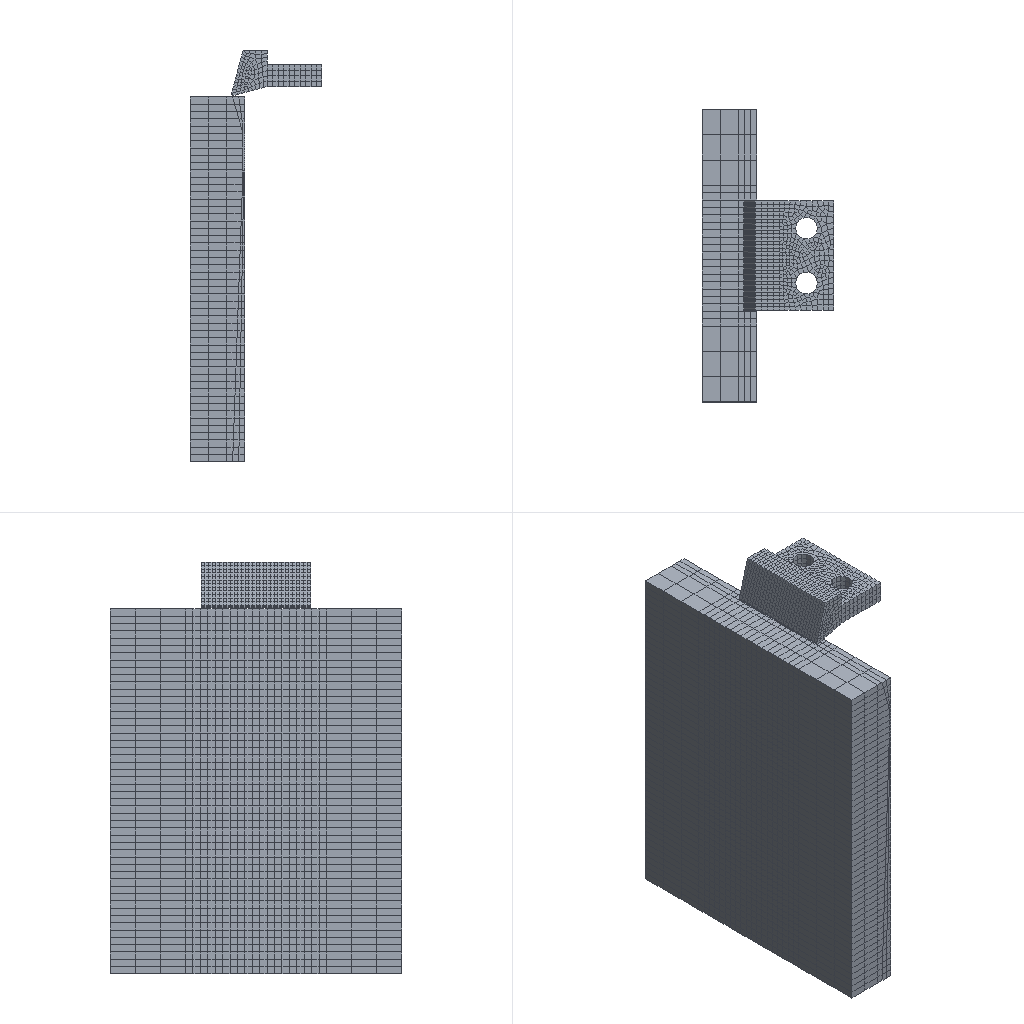Simulation study | abaqus
Set-up summary:
category,name,step,type,value,unit,region
solver,abaqus
solver,version,,,Abaqus/Explicit 2020
units,not stated in the deck,,not stated
analysis,deck,,transient,transient
load_step,Step-1,Step-1,transient
load_step,requested,,,1
mesh,nodes,,,19292
mesh,elements,,,12938
element_type,C3D8,,solid,3738
element_type,C3D8R,,solid,9200
load,load commands in deck,,count,1
bc,support commands in deck,,count,8
material,Q345,,in results
material,SLPSB,,in results
material,SLPSB2,,in results
material,SOIL,,in results
material,SOIL-COPY,,in results
check,setup vs results,,match,"per instance, exact: element labels, types and connectivity; labels of the nodes the elements use; coordinates of those nodes at DOUBLE_PRECISION in 1 of 3 instance(s)"
Abaqus input file, long lists of numbers shortened:
*Heading
** Job name: retiaoshi Model name: Model-1
** Generated by: Abaqus/CAE 2020
*Preprint, echo=NO, model=NO, history=NO, contact=NO
**
** PARTS
**
*Part, name=newwork
*Node
      1,           0.,  -59.32,         -20.
      2,         14.5,  -59.32,         -20.
** (7746 more lines like these left out)
*Element, type=C3D8R
 1,   74,  855, 3789,  839,    1,   53,  831,   59
 2,  855,  856, 3790, 3789,   53,   54,  832,  831
** (5998 more lines like these left out)
*Nset, nset=Set-7, generate
    1,  7748,     1
*Elset, elset=Set-7, generate
    1,  6000,     1
*Nset, nset=tuchipaa
   89,   90,   91,   92,   93,   94,   95,   96,   97,   98,   99,  100,  101,  102,  103,  104
  105,  106,  127,  128,  129,  130,  131,  132,  133,  134,  135,  136,  137,  138,  139,  140
** (219 more lines like these left out)
*Nset, nset=cc1
    4,    9,   16,   29,   30,   34,   43,   51,   56,   63,  172,  173,  545,  546,  559,  560
  603,  626,  709,  755, 1092, 3189, 3285, 3566
*Elset, elset=_tuti_S1, internal, generate
 4761,  4775,     1
*Elset, elset=_tuti_S4, internal, generate
  3,  45,   3
*Surface, type=ELEMENT, name=tuti
_tuti_S1, S1
_tuti_S4, S4
*Elset, elset=_m1_S1, internal, generate
 4761,  4775,     1
*Elset, elset=_m1_S4, internal, generate
  3,  45,   3
*Surface, type=ELEMENT, name=m1
_m1_S1, S1
_m1_S4, S4
** Section: tuti
*Solid Section, elset=Set-7, material=soil
,
*End Part
**
*Part, name=qiedao
*Node
      1,           3.,   7.052,           0.
      2,          -3.,   7.052,           0.
** (4779 more lines like these left out)
*Element, type=C3D8
   1,  408,  428,  429,  410, 2071, 2091, 2092, 2073
   2,   42,   41,    5,    6, 1026, 1027,  196,  138
** (3736 more lines like these left out)
*Node
   4782, 1.55431223e-15,   7.052,          15.
*Nset, nset=qiedao-RefPt_, internal
4782,
*Nset, nset=_PickedSet2, internal, generate
    1,  4781,     1
*Elset, elset=_PickedSet2, internal, generate
    1,  3738,     1
*Nset, nset=Set-daoju, generate
    1,  4782,     1
*Elset, elset=Set-daoju, generate
    1,  3738,     1
*Elset, elset=ganggang
    1,    2,    3,    4,    5,    6,    7,    8,    9,   10,   11,   12,   13,   14,   15,   16
   17,   18,   19,   20,   21,   22,   23,   24,   25,   26,   27,   28,   29,   30,   31,   32
** (104 more lines like these left out)
*Elset, elset=_keng-dao_S1, internal
    1,    2,    3,    4,    5,    6,    7,    8,    9,   10,   11,   12,   13,   14,   15,   16
   17,   18,   19,   20,   21,   22,   23,   24,   25,   26,   27,   28,   29,   30,   31,   32
** (22 more lines like these left out)
*Elset, elset=_keng-dao_S2, internal
 2524, 2525, 2526, 2527, 2528, 2529, 2530, 2531, 2532, 2533, 2534, 2535, 2536, 2537, 2538, 2539
 2540, 2541, 2542, 2543, 2544, 2545, 2546, 2547, 2548, 2549, 2550, 2551, 2552, 2553, 2554, 2555
** (22 more lines like these left out)
*Elset, elset=_keng-dao_S3, internal
    2,    5,    7,   10,   11,   12,   13,   16,   18,   21,   27,   28,   36,   89,   92,   94
   97,   98,   99,  100,  103,  105,  108,  114,  115,  123,  176,  179,  181,  184,  185,  186
** (29 more lines like these left out)
*Elset, elset=_keng-dao_S4, internal
    2,   89,  176,  263,  350,  437,  524,  611,  698,  785,  872,  959, 1046, 1133, 1220, 1307
 1394, 1481, 1568, 1655, 1742, 1829, 1916, 2003, 2090, 2177, 2264, 2351, 2438, 2525, 2640, 2722
** (3 more lines like these left out)
*Elset, elset=_keng-dao_S5, internal
    3,    8,   14,   15,   17,   19,   25,   29,   30,   31,   39,   41,   42,   44,   90,   95
  101,  102,  104,  106,  112,  116,  117,  118,  126,  128,  129,  131,  177,  182,  188,  189
** (30 more lines like these left out)
*Elset, elset=_keng-dao_S6, internal
    2,    8,   22,   84,   89,   95,  109,  171,  176,  182,  196,  258,  263,  269,  283,  345
  350,  356,  370,  432,  437,  443,  457,  519,  524,  530,  544,  606,  611,  617,  631,  693
** (9 more lines like these left out)
*Surface, type=ELEMENT, name=keng-dao
_keng-dao_S1, S1
_keng-dao_S2, S2
_keng-dao_S4, S4
_keng-dao_S6, S6
_keng-dao_S3, S3
_keng-dao_S5, S5
** Section: Q345
*Solid Section, elset=_PickedSet2, material=q345
,
*End Part
**
*Part, name=suliao
*Node
      1,           0.,         -80.,         -10.
      2,           0.,        -79.5,         -10.
** (6760 more lines like these left out)
*Element, type=C3D8R
   1,  323,  324,  485,  484,    1,    2,  163,  162
   2,  324,  325,  486,  485,    2,    3,  164,  163
** (3198 more lines like these left out)
*Nset, nset=Set-3, generate
    1,  6762,     1
*Elset, elset=Set-3, generate
    1,  3200,     1
*Nset, nset=suchipaa
   45,   46,   47,   48,   49,   50,   51,   52,   53,   54,   55,   56,   57,   58,   59,   60
   61,   62,   63,   64,   65,   66,   67,   68,   69,   70,   71,   72,   73,   74,   75,   76
** (166 more lines like these left out)
*Nset, nset=m2
    1,    2,    3,    4,    5,    6,    7,    8,    9,   10,   11,   12,   13,   14,   15,   16
   17,   18,   19,  140,  141,  142,  143,  144,  145,  146,  147,  148,  149,  150,  151,  152
** (51 more lines like these left out)
*Nset, nset=ce1
   1,   2,   3,   4,   5,   6,   7,   8,   9, 151, 152, 153, 154, 155, 156, 157
 158, 159, 160, 161, 162, 163, 164, 165, 166, 167, 168, 169, 170, 312, 313, 314
** (1 more lines like these left out)
*Nset, nset=ce2
 6441, 6442, 6443, 6444, 6445, 6446, 6447, 6448, 6449, 6592, 6593, 6594, 6595, 6596, 6597, 6598
 6599, 6600, 6601, 6602, 6603, 6604, 6605, 6606, 6607, 6608, 6609, 6610, 6753, 6754, 6755, 6756
** (1 more lines like these left out)
*Elset, elset=_suliaoban_S3, internal, generate
    1,  3200,     1
*Surface, type=ELEMENT, name=suliaoban
_suliaoban_S3, S3
** Section: suliaoti
*Solid Section, elset=Set-3, material=slpsb
,
*End Part
**
**
** ASSEMBLY
**
*Assembly, name=Assembly
**
*Instance, name=qiedao-1, part=qiedao
   28.199,         -55., 5.826
   28.199,         -55., 5.826, 27.621, -54.423, 6.403,         120.
*End Instance
**
*Instance, name=newwork-1, part=newwork
*End Instance
**
*Instance, name=suliao-1, part=suliao
        14.5,           0.,         -10.
*End Instance
**
*Nset, nset=Set-20, instance=qiedao-1
 4782,
*Nset, nset=Set-25, instance=suliao-1
    1,  161,  162,  322,  323,  483,  484,  644,  645,  805,  806,  966,  967, 1127, 1128, 1288
 1289, 1449, 1450, 1610, 1611, 1771, 1772, 1932, 1933, 2093, 2094, 2254, 2255, 2415, 2416, 2576
** (4 more lines like these left out)
*Elset, elset=Set-25, instance=suliao-1
    1,  160,  161,  320,  321,  480,  481,  640,  641,  800,  801,  960,  961, 1120, 1121, 1280
 1281, 1440, 1441, 1600, 1601, 1760, 1761, 1920, 1921, 2080, 2081, 2240, 2241, 2400, 2401, 2560
** (1 more lines like these left out)
*Nset, nset=Set-26, instance=newwork-1
    1,    5,    6,   10,   11,   13,   21,   22,   26,   27,   28,   39,   40,   42,   47,   50
   58,   59,   65,   66,   67,   68,   69,   70,   71,   72,   73,   74,  107,  108,  109,  110
** (81 more lines like these left out)
*Elset, elset=Set-26, instance=newwork-1
    1,    4,    7,   10,   13,   16,   19,   22,   25,   28,   31,   34,   37,   40,   43,   46
   49,   52,   55,   58,   61,   64,   67,   70,   73,   76,   79,   82,   85,   88,   91,   94
** (77 more lines like these left out)
*Nset, nset=_PickedSet56, internal, instance=qiedao-1
 4782,
*Surface, type=NODE, name=newwork-1_tuchipaa_CNS_, internal
newwork-1.tuchipaa, 1.
*Surface, type=NODE, name=suliao-1_suchipaa_CNS_, internal
suliao-1.suchipaa, 1.
*Surface, type=NODE, name=suliao-1_ce1_CNS_, internal
suliao-1.ce1, 1.
*Surface, type=NODE, name=newwork-1_cc1_CNS_, internal
newwork-1.cc1, 1.
*Surface, type=NODE, name=suliao-1_ce2_CNS_, internal
suliao-1.ce2, 1.
** Constraint: Constraint-1
*Rigid Body, ref node=_PickedSet56, elset=qiedao-1.ganggang
** Constraint: Constraint-4
*Tie, name=Constraint-4, adjust=yes, type=NODE TO SURFACE
newwork-1_cc1_CNS_, suliao-1_ce1_CNS_
** Constraint: Constraint-5
*Tie, name=Constraint-5, adjust=yes, type=NODE TO SURFACE
newwork-1_cc1_CNS_, suliao-1_ce2_CNS_
*End Assembly
**
** MATERIALS
**
*Material, name=q345
*Density
 7.85e-09,
*Elastic
206000., 0.3
*Material, name=slpsb
*Damage Initiation, criterion=SHEAR
 0.1,0.,0.
*Damage Evolution, type=DISPLACEMENT
 0.05,
*Density
 1.2e-09,
*Elastic
890000., 0.42
*Plastic
   0.001,        0.
 19.066,  0.02392
 29.961, 0.03986
 38.132, 0.05393
 49.027, 0.07081
 100.778, 0.09335
 147.082,   0.1084
 198.833,  0.1192
 242.412,  0.1277
 299.611,  0.1357
 345.914,  0.1423
 397.665,  0.1479
 446.693,  0.1559
  495.72,  0.1639
 542.023,  0.1691
 593.774,  0.1748
*Material, name=slpsb2
*Damage Initiation, criterion=SHEAR
 0.5,   0.33, 0.0001
*Damage Evolution, type=DISPLACEMENT
 0.5,
*Density
 1.88e-09,
*Elastic
 10.9, 0.35
*Plastic
   0.001,        0.
 19.066,  0.02392
 29.961, 0.03986
 38.132, 0.05393
 49.027, 0.07081
 100.778, 0.09335
 147.082,   0.1084
 198.833,  0.1192
 242.412,  0.1277
 299.611,  0.1357
 345.914,  0.1423
 397.665,  0.1479
 446.693,  0.1559
  495.72,  0.1639
 542.023,  0.1691
 593.774,  0.1748
*Material, name=soil
*Damage Initiation, criterion=SHEAR
 0.007,0.,0.
*Damage Evolution, type=DISPLACEMENT
 0.007,
*Density
 1.88e-09,
*Drucker Prager
35., 0.885,   29.
*Drucker Prager Hardening
10.,0.
*Elastic
 10.9, 0.35
*Material, name=soil-Copy
*Damage Initiation, criterion=SHEAR
 0.5,   0.33, 0.0001
*Damage Evolution, type=DISPLACEMENT
 0.03,
*Density
 1.88e-09,
*Elastic
 10.9, 0.35
*Plastic
 9.,   0.
12., 0.02
15., 0.04
17., 0.06
18., 0.08
19.,  0.1
20., 0.12
**
** INTERACTION PROPERTIES
**
*Surface Interaction, name=IntProp-1
*Friction
 0.3,
*Surface Behavior, pressure-overclosure=HARD
**
** BOUNDARY CONDITIONS
**
** Name: BC-3 Type: 对称/反对称/完全固定
*Boundary
Set-25, ENCASTRE
** Name: BC-7 Type: 对称/反对称/完全固定
*Boundary
Set-26, ENCASTRE
** ----------------------------------------------------------------
**
** STEP: Step-1
**
*Step, name=Step-1, nlgeom=YES
*Dynamic, Explicit
, 1.6
*Bulk Viscosity
0.06, 1.2
** Mass Scaling: Semi-Automatic
**               Whole Model
*Fixed Mass Scaling, dt=1e-05, type=below min
**
** BOUNDARY CONDITIONS
**
** Name: jingei Type: Velocity/Angular velocity
*Boundary, type=VELOCITY
Set-20, 1, 1
Set-20, 2, 2
Set-20, 3, 3, -80.
Set-20, 4, 4
Set-20, 5, 5
Set-20, 6, 6
*Adaptive Mesh Controls, name=Ada-1
1., 0., 0.
**
** INTERACTIONS
**
** Interaction: Int-1
*Contact Pair, interaction=IntProp-1, mechanical constraint=KINEMATIC, cpset=Int-1
qiedao-1.keng-dao, newwork-1_tuchipaa_CNS_
** Interaction: Int-2
*Contact Pair, interaction=IntProp-1, mechanical constraint=KINEMATIC, cpset=Int-2
qiedao-1.keng-dao, suliao-1_suchipaa_CNS_
**
** OUTPUT REQUESTS
**
*Restart, write, number interval=1, time marks=NO
**
** FIELD OUTPUT: F-Output-1
**
*Output, field, number interval=200
*Node Output
A, RF, RT, U, V
*Element Output, directions=YES
LE, MISES, PE, PEEQ, PEEQVAVG, PEVAVG, S, STATUS
*Contact Output
CSTRESS,
**
** HISTORY OUTPUT: H-Output-1
**
*Output, history, variable=PRESELECT
*End Step
Results summary:
result,step,Step-1,completed,increments=385904 time=1.6/1.6
result,analysis,,,transient
result,last_loadstep,,,1
result,primary field,,,U
result,reaction total,,FX,0.08034,model units
result,reaction total,,FY,35.775,model units
result,reaction total,,FZ,62.391,model units